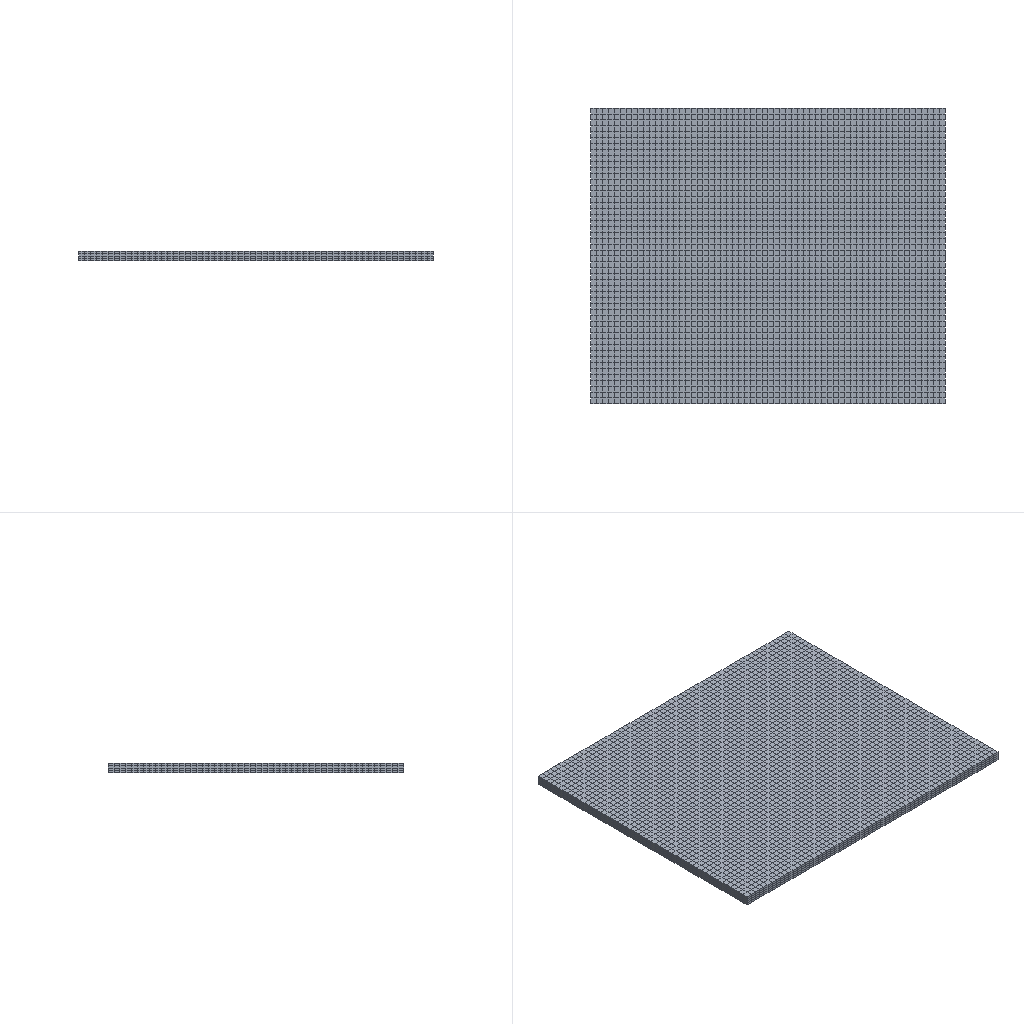Simulation study | abaqus
Set-up summary:
category,name,step,type,value,unit,region
solver,abaqus
solver,version,,,Abaqus/Explicit 2020
units,not stated in the deck,,not stated
analysis,deck,,transient,transient
load_step,Step-1,Step-1,transient
load_step,requested,,,1
mesh,nodes,,,23024
mesh,elements,,,19907
element_type,R3D3,,rigid,888
element_type,R3D4,,rigid,7019
element_type,C3D8R,,solid,12000
load,load commands in deck,,count,1
bc,support commands in deck,,count,9
material,MATERIAL-1,,in results
check,setup vs results,,match,"per instance, exact: element labels, types and connectivity; labels of the nodes the elements use; coordinates of those nodes at SINGLE_PRECISION in 3 of 3 instance(s)"
Abaqus input file, long lists of numbers shortened:
*Heading
** Job name: Job-1 Model name: Model-1
** Generated by: Abaqus/CAE 2020
*Preprint, echo=NO, model=NO, history=NO, contact=NO
**
** PARTS
**
*Part, name=maopi
*Node
      1,           0.,       -1500.,          50.
      2,           0.,       -1470.,          50.
** (15553 more lines like these left out)
*Element, type=C3D8R
    1,   256,   257,   308,   307,     1,     2,    53,    52
    2,   257,   258,   309,   308,     2,     3,    54,    53
** (11998 more lines like these left out)
*Nset, nset=Set-1, generate
     1,  15555,      1
*Elset, elset=Set-1, generate
     1,  12000,      1
** Section: Section-1
*Solid Section, elset=Set-1, material=Material-1
,
*End Part
**
*Part, name=work-88
*Node
      1,   816.527,  -590.876,   152.301
      2,   816.527,   572.254,   152.301
** (4022 more lines like these left out)
*Element, type=R3D4
   1,    1,  347, 1295,  482
   2,  347,  348, 1296, 1295
** (3807 more lines like these left out)
*Element, type=R3D3
1920, 2706,  485,  484
1921, 2708, 2709, 2705
** (424 more lines like these left out)
*Node
   4025, 1.98951966e-11,  -9.311,   152.301
*Nset, nset=work-88-RefPt_, internal
4025,
*Elset, elset=work-88, generate
    1,  4235,     1
*End Part
**
*Part, name=work-90
*Node
      1,  -766.527,  -490.876,   13.185
      2,  -766.527,  -490.876,  -38.918
** (3441 more lines like these left out)
*Element, type=R3D4
1,   1,   2, 347, 348
2, 348, 347,   3,   4
** (3208 more lines like these left out)
*Element, type=R3D3
481, 1699, 1875, 1700
482, 1952, 1880, 1874
** (460 more lines like these left out)
*Node
   3444, -7.10542736e-15,  -9.311,  -38.918
*Nset, nset=work-90-RefPt_, internal
3444,
*Elset, elset=work-90, generate
    1,  3672,     1
*End Part
**
**
** ASSEMBLY
**
*Assembly, name=Assembly
**
*Instance, name=work-90-1, part=work-90
          0.,           0.,        -170.
*End Instance
**
*Instance, name=work-88-1, part=work-88
*End Instance
**
*Instance, name=maopi-1, part=maopi
 -886.527,   722.254,   -79.461
*End Instance
**
*Nset, nset=Set-1, instance=work-88-1
 4025,
*Nset, nset=Set-2, instance=work-90-1
 3444,
*Nset, nset=Set-3, instance=maopi-1
     1,    51,    52,   102,   103,   153,   154,   204,   205,   255,   256,   306,   307,   357,   358,   408
   409,   459,   460,   510,   511,   561,   562,   612,   613,   663,   664,   714,   715,   765,   766,   816
** (37 more lines like these left out)
*Elset, elset=Set-3, instance=maopi-1
     1,    50,    51,   100,   101,   150,   151,   200,   201,   250,   251,   300,   301,   350,   351,   400
   401,   450,   451,   500,   501,   550,   551,   600,   601,   650,   651,   700,   701,   750,   751,   800
** (28 more lines like these left out)
*Nset, nset=Set-4, instance=maopi-1
     1,     2,     3,     4,     5,     6,     7,     8,     9,    10,    11,    12,    13,    14,    15,    16
    17,    18,    19,    20,    21,    22,    23,    24,    25,    26,    27,    28,    29,    30,    31,    32
** (30 more lines like these left out)
*Elset, elset=Set-4, instance=maopi-1
     1,     2,     3,     4,     5,     6,     7,     8,     9,    10,    11,    12,    13,    14,    15,    16
    17,    18,    19,    20,    21,    22,    23,    24,    25,    26,    27,    28,    29,    30,    31,    32
** (23 more lines like these left out)
*Rigid Body, ref node=work-90-1.work-90-RefPt_, elset=work-90-1.work-90
*Rigid Body, ref node=work-88-1.work-88-RefPt_, elset=work-88-1.work-88
*End Assembly
*Amplitude, name=Amp-1
             0.,              0.,            0.01,              1.
**
** MATERIALS
**
*Material, name=Material-1
*Density
 2.7e-09,
*Elastic
72000., 0.3
*Plastic
300.,0.
**
** INTERACTION PROPERTIES
**
*Surface Interaction, name=IntProp-1
*Friction
 0.1,
*Surface Behavior, pressure-overclosure=HARD
**
** BOUNDARY CONDITIONS
**
** Name: BC-1 Type: 对称/反对称/完全固定
*Boundary
Set-1, ENCASTRE
** ----------------------------------------------------------------
**
** STEP: Step-1
**
*Step, name=Step-1, nlgeom=YES
*Dynamic, Explicit
, 0.01
*Bulk Viscosity
0.06, 1.2
** Mass Scaling: Semi-Automatic
**               Whole Model
*Fixed Mass Scaling, factor=500.
**
** BOUNDARY CONDITIONS
**
** Name: BC-3 Type: 位移/转角
*Boundary
Set-3, 2, 2
** Name: BC-4 Type: 位移/转角
*Boundary
Set-4, 1, 1
** Name: [REDACTED] : Displacement/rotation angle
*Boundary, amplitude=Amp-1
Set-2, 1, 1
Set-2, 2, 2
Set-2, 3, 3, 150.
Set-2, 4, 4
Set-2, 5, 5
Set-2, 6, 6
**
** INTERACTIONS
**
** Interaction: Int-1
*Contact, op=NEW
*Contact Inclusions, ALL EXTERIOR
*Contact Property Assignment
 ,  , IntProp-1
**
** OUTPUT REQUESTS
**
*Restart, write, number interval=1, time marks=NO
**
** FIELD OUTPUT: F-Output-1
**
*Output, field, number interval=50
*Node Output
A, RF, RM, RT, U, V
*Element Output, directions=YES
E, EVF, LE, MISES, MISESMAX, PE, PEEQ, PEEQVAVG, PEVAVG, S, SVAVG
*Contact Output
CDISP, CSTRESS
**
** HISTORY OUTPUT: H-Output-1
**
*Output, history, variable=PRESELECT
*End Step
Results summary:
result,step,Step-1,completed,increments=306 time=0.01/0.01
result,analysis,,,transient
result,last_loadstep,,,1
result,primary field,,,U
result,reaction total,,FX,21215599.125,model units
result,reaction total,,FY,-15691174.303,model units
result,reaction total,,FZ,2028079104.0,model units